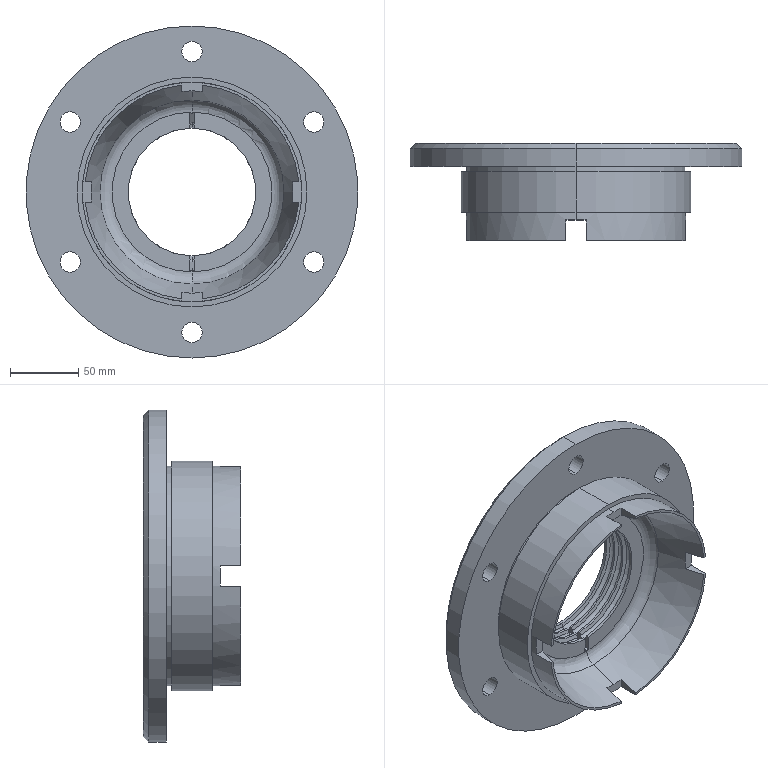Part | SolidWorks | features ICE 3, Fillet 1, RevCut 1, Revolution 1, Scale 1 | 1 solid | 80 faces | box 243.75 x 71.25 x 243.75 mm | volume 1007577 mm3 | cylinder 28 | plane 25 | cone 19 | torus 8 | commonest cylinder face diameters 15 x12 93.75 x8 161.25 x4 168.75 x2 243.75 x2